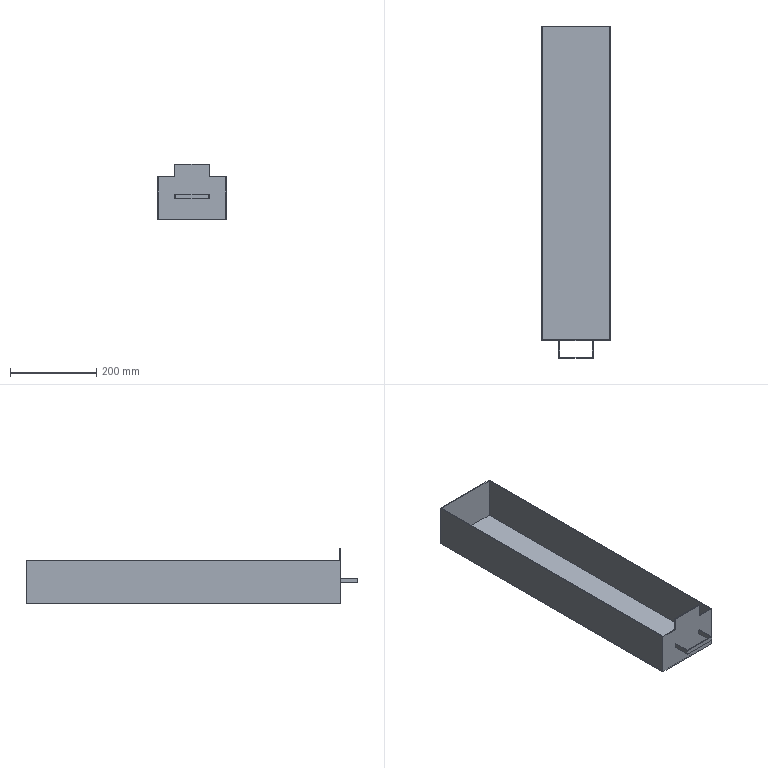Part | NX | features solid 2 | 1 solid | 22 faces | box 160 x 772 x 130 mm | volume 590256 mm3 | plane 22
STEP:
#1=CARTESIAN_POINT('',(-175.,-255.,-465.));
#2=VERTEX_POINT('',#1);
#3=CARTESIAN_POINT('',(-175.,-987.,-465.));
#4=VERTEX_POINT('',#3);
#5=CARTESIAN_POINT('',(-175.,-687.,-465.));
#6=DIRECTION('',(0.,-1.,0.));
#7=VECTOR('',#6,1000.);
#8=LINE('',#5,#7);
#9=EDGE_CURVE('',#2,#4,#8,.T.);
#10=ORIENTED_EDGE('',*,*,#9,.T.);
#11=CARTESIAN_POINT('',(-175.,-987.,-565.));
#12=VERTEX_POINT('',#11);
#13=CARTESIAN_POINT('',(-175.,-987.,-565.));
#14=DIRECTION('',(0.,0.,1.));
#15=VECTOR('',#14,1000.);
#16=LINE('',#13,#15);
#17=EDGE_CURVE('',#12,#4,#16,.T.);
#18=ORIENTED_EDGE('',*,*,#17,.F.);
#19=CARTESIAN_POINT('',(-175.,-255.,-565.));
#20=VERTEX_POINT('',#19);
#21=CARTESIAN_POINT('',(-175.,-687.,-565.));
#22=DIRECTION('',(0.,-1.,0.));
#23=VECTOR('',#22,1000.);
#24=LINE('',#21,#23);
#25=EDGE_CURVE('',#20,#12,#24,.T.);
#26=ORIENTED_EDGE('',*,*,#25,.F.);
#27=CARTESIAN_POINT('',(-175.,-255.,-565.));
#28=DIRECTION('',(0.,0.,-1.));
#29=VECTOR('',#28,1000.);
#30=LINE('',#27,#29);
#31=EDGE_CURVE('',#20,#2,#30,.F.);
#32=ORIENTED_EDGE('',*,*,#31,.T.);
#33=EDGE_LOOP('',(#10,#18,#26,#32));
#34=FACE_BOUND('',#33,.T.);
#35=CARTESIAN_POINT('',(-175.,-687.,-565.));
#36=DIRECTION('',(-1.,0.,0.));
#37=DIRECTION('',(0.,-1.,0.));
#38=AXIS2_PLACEMENT_3D('',#35,#36,#37);
#39=PLANE('',#38);
#40=ADVANCED_FACE('',(#34),#39,.F.);
#41=CARTESIAN_POINT('',(-295.,-987.,-505.));
#42=VERTEX_POINT('',#41);
#43=CARTESIAN_POINT('',(-295.,-987.,-515.));
#44=VERTEX_POINT('',#43);
#45=CARTESIAN_POINT('',(-295.,-987.,-565.));
#46=DIRECTION('',(0.,0.,-1.));
#47=VECTOR('',#46,1000.);
#48=LINE('',#45,#47);
#49=EDGE_CURVE('',#42,#44,#48,.T.);
#50=ORIENTED_EDGE('',*,*,#49,.F.);
#51=CARTESIAN_POINT('',(-293.,-987.,-505.));
#52=VERTEX_POINT('',#51);
#53=CARTESIAN_POINT('',(-215.,-987.,-505.));
#54=DIRECTION('',(1.,0.,0.));
#55=VECTOR('',#54,1000.);
#56=LINE('',#53,#55);
#57=EDGE_CURVE('',#52,#42,#56,.F.);
#58=ORIENTED_EDGE('',*,*,#57,.F.);
#59=CARTESIAN_POINT('',(-293.,-987.,-515.));
#60=VERTEX_POINT('',#59);
#61=CARTESIAN_POINT('',(-293.,-987.,-565.));
#62=DIRECTION('',(0.,0.,-1.));
#63=VECTOR('',#62,1000.);
#64=LINE('',#61,#63);
#65=EDGE_CURVE('',#52,#60,#64,.T.);
#66=ORIENTED_EDGE('',*,*,#65,.T.);
#67=CARTESIAN_POINT('',(-215.,-987.,-515.));
#68=DIRECTION('',(1.,0.,0.));
#69=VECTOR('',#68,1000.);
#70=LINE('',#67,#69);
#71=EDGE_CURVE('',#60,#44,#70,.F.);
#72=ORIENTED_EDGE('',*,*,#71,.T.);
#73=EDGE_LOOP('',(#50,#58,#66,#72));
#74=FACE_BOUND('',#73,.T.);
#75=CARTESIAN_POINT('',(-217.,-987.,-505.));
#76=VERTEX_POINT('',#75);
#77=CARTESIAN_POINT('',(-217.,-987.,-515.));
#78=VERTEX_POINT('',#77);
#79=CARTESIAN_POINT('',(-217.,-987.,-565.));
#80=DIRECTION('',(0.,0.,1.));
#81=VECTOR('',#80,1000.);
#82=LINE('',#79,#81);
#83=EDGE_CURVE('',#76,#78,#82,.F.);
#84=ORIENTED_EDGE('',*,*,#83,.F.);
#85=CARTESIAN_POINT('',(-215.,-987.,-505.));
#86=VERTEX_POINT('',#85);
#87=CARTESIAN_POINT('',(-215.,-987.,-505.));
#88=DIRECTION('',(1.,0.,0.));
#89=VECTOR('',#88,1000.);
#90=LINE('',#87,#89);
#91=EDGE_CURVE('',#86,#76,#90,.F.);
#92=ORIENTED_EDGE('',*,*,#91,.F.);
#93=CARTESIAN_POINT('',(-215.,-987.,-515.));
#94=VERTEX_POINT('',#93);
#95=CARTESIAN_POINT('',(-215.,-987.,-565.));
#96=DIRECTION('',(0.,0.,-1.));
#97=VECTOR('',#96,1000.);
#98=LINE('',#95,#97);
#99=EDGE_CURVE('',#86,#94,#98,.T.);
#100=ORIENTED_EDGE('',*,*,#99,.T.);
#101=CARTESIAN_POINT('',(-215.,-987.,-515.));
#102=DIRECTION('',(1.,0.,0.));
#103=VECTOR('',#102,1000.);
#104=LINE('',#101,#103);
#105=EDGE_CURVE('',#94,#78,#104,.F.);
#106=ORIENTED_EDGE('',*,*,#105,.T.);
#107=EDGE_LOOP('',(#84,#92,#100,#106));
#108=FACE_BOUND('',#107,.T.);
#109=CARTESIAN_POINT('',(-335.,-987.,-465.));
#110=VERTEX_POINT('',#109);
#111=CARTESIAN_POINT('',(-295.,-987.,-465.));
#112=VERTEX_POINT('',#111);
#113=CARTESIAN_POINT('',(-180.,-987.,-465.));
#114=DIRECTION('',(1.,0.,0.));
#115=VECTOR('',#114,1000.);
#116=LINE('',#113,#115);
#117=EDGE_CURVE('',#110,#112,#116,.T.);
#118=ORIENTED_EDGE('',*,*,#117,.F.);
#119=CARTESIAN_POINT('',(-335.,-987.,-565.));
#120=VERTEX_POINT('',#119);
#121=CARTESIAN_POINT('',(-335.,-987.,-565.));
#122=DIRECTION('',(0.,0.,-1.));
#123=VECTOR('',#122,1000.);
#124=LINE('',#121,#123);
#125=EDGE_CURVE('',#120,#110,#124,.F.);
#126=ORIENTED_EDGE('',*,*,#125,.F.);
#127=CARTESIAN_POINT('',(-180.,-987.,-565.));
#128=DIRECTION('',(-1.,0.,0.));
#129=VECTOR('',#128,1000.);
#130=LINE('',#127,#129);
#131=EDGE_CURVE('',#12,#120,#130,.T.);
#132=ORIENTED_EDGE('',*,*,#131,.F.);
#133=ORIENTED_EDGE('',*,*,#17,.T.);
#134=CARTESIAN_POINT('',(-215.,-987.,-465.));
#135=VERTEX_POINT('',#134);
#136=CARTESIAN_POINT('',(-180.,-987.,-465.));
#137=DIRECTION('',(1.,0.,0.));
#138=VECTOR('',#137,1000.);
#139=LINE('',#136,#138);
#140=EDGE_CURVE('',#135,#4,#139,.T.);
#141=ORIENTED_EDGE('',*,*,#140,.F.);
#142=CARTESIAN_POINT('',(-215.,-987.,-435.));
#143=VERTEX_POINT('',#142);
#144=CARTESIAN_POINT('',(-215.,-987.,-565.));
#145=DIRECTION('',(0.,0.,1.));
#146=VECTOR('',#145,1000.);
#147=LINE('',#144,#146);
#148=EDGE_CURVE('',#135,#143,#147,.T.);
#149=ORIENTED_EDGE('',*,*,#148,.T.);
#150=CARTESIAN_POINT('',(-295.,-987.,-435.));
#151=VERTEX_POINT('',#150);
#152=CARTESIAN_POINT('',(-175.,-987.,-435.));
#153=DIRECTION('',(-1.,0.,0.));
#154=VECTOR('',#153,1000.);
#155=LINE('',#152,#154);
#156=EDGE_CURVE('',#143,#151,#155,.T.);
#157=ORIENTED_EDGE('',*,*,#156,.T.);
#158=CARTESIAN_POINT('',(-295.,-987.,-565.));
#159=DIRECTION('',(0.,0.,-1.));
#160=VECTOR('',#159,1000.);
#161=LINE('',#158,#160);
#162=EDGE_CURVE('',#112,#151,#161,.F.);
#163=ORIENTED_EDGE('',*,*,#162,.F.);
#164=EDGE_LOOP('',(#118,#126,#132,#133,#141,#149,#157,#163));
#165=FACE_BOUND('',#164,.T.);
#166=CARTESIAN_POINT('',(-180.,-987.,-565.));
#167=DIRECTION('',(0.,1.,0.));
#168=DIRECTION('',(-1.,0.,0.));
#169=AXIS2_PLACEMENT_3D('',#166,#167,#168);
#170=PLANE('',#169);
#171=ADVANCED_FACE('',(#74,#108,#165),#170,.F.);
#172=ORIENTED_EDGE('',*,*,#125,.T.);
#173=CARTESIAN_POINT('',(-335.,-255.,-465.));
#174=VERTEX_POINT('',#173);
#175=CARTESIAN_POINT('',(-335.,-687.,-465.));
#176=DIRECTION('',(0.,1.,0.));
#177=VECTOR('',#176,1000.);
#178=LINE('',#175,#177);
#179=EDGE_CURVE('',#174,#110,#178,.F.);
#180=ORIENTED_EDGE('',*,*,#179,.F.);
#181=CARTESIAN_POINT('',(-335.,-255.,-565.));
#182=VERTEX_POINT('',#181);
#183=CARTESIAN_POINT('',(-335.,-255.,-565.));
#184=DIRECTION('',(0.,0.,1.));
#185=VECTOR('',#184,1000.);
#186=LINE('',#183,#185);
#187=EDGE_CURVE('',#182,#174,#186,.T.);
#188=ORIENTED_EDGE('',*,*,#187,.F.);
#189=CARTESIAN_POINT('',(-335.,-687.,-565.));
#190=DIRECTION('',(0.,1.,0.));
#191=VECTOR('',#190,1000.);
#192=LINE('',#189,#191);
#193=EDGE_CURVE('',#182,#120,#192,.F.);
#194=ORIENTED_EDGE('',*,*,#193,.T.);
#195=EDGE_LOOP('',(#172,#180,#188,#194));
#196=FACE_BOUND('',#195,.T.);
#197=CARTESIAN_POINT('',(-335.,-687.,-565.));
#198=DIRECTION('',(-1.,0.,0.));
#199=DIRECTION('',(0.,-1.,0.));
#200=AXIS2_PLACEMENT_3D('',#197,#198,#199);
#201=PLANE('',#200);
#202=ADVANCED_FACE('',(#196),#201,.T.);
#203=CARTESIAN_POINT('',(-333.,-985.,-563.));
#204=VERTEX_POINT('',#203);
#205=CARTESIAN_POINT('',(-333.,-985.,-465.));
#206=VERTEX_POINT('',#205);
#207=CARTESIAN_POINT('',(-333.,-985.,-565.));
#208=DIRECTION('',(0.,0.,-1.));
#209=VECTOR('',#208,1000.);
#210=LINE('',#207,#209);
#211=EDGE_CURVE('',#204,#206,#210,.F.);
#212=ORIENTED_EDGE('',*,*,#211,.T.);
#213=CARTESIAN_POINT('',(-295.,-985.,-465.));
#214=VERTEX_POINT('',#213);
#215=CARTESIAN_POINT('',(-180.,-985.,-465.));
#216=DIRECTION('',(1.,0.,0.));
#217=VECTOR('',#216,1000.);
#218=LINE('',#215,#217);
#219=EDGE_CURVE('',#206,#214,#218,.T.);
#220=ORIENTED_EDGE('',*,*,#219,.T.);
#221=CARTESIAN_POINT('',(-295.,-985.,-435.));
#222=VERTEX_POINT('',#221);
#223=CARTESIAN_POINT('',(-295.,-985.,-565.));
#224=DIRECTION('',(0.,0.,-1.));
#225=VECTOR('',#224,1000.);
#226=LINE('',#223,#225);
#227=EDGE_CURVE('',#214,#222,#226,.F.);
#228=ORIENTED_EDGE('',*,*,#227,.T.);
#229=CARTESIAN_POINT('',(-215.,-985.,-435.));
#230=VERTEX_POINT('',#229);
#231=CARTESIAN_POINT('',(-175.,-985.,-435.));
#232=DIRECTION('',(-1.,0.,0.));
#233=VECTOR('',#232,1000.);
#234=LINE('',#231,#233);
#235=EDGE_CURVE('',#230,#222,#234,.T.);
#236=ORIENTED_EDGE('',*,*,#235,.F.);
#237=CARTESIAN_POINT('',(-215.,-985.,-465.));
#238=VERTEX_POINT('',#237);
#239=CARTESIAN_POINT('',(-215.,-985.,-565.));
#240=DIRECTION('',(0.,0.,1.));
#241=VECTOR('',#240,1000.);
#242=LINE('',#239,#241);
#243=EDGE_CURVE('',#238,#230,#242,.T.);
#244=ORIENTED_EDGE('',*,*,#243,.F.);
#245=CARTESIAN_POINT('',(-177.,-985.,-465.));
#246=VERTEX_POINT('',#245);
#247=CARTESIAN_POINT('',(-180.,-985.,-465.));
#248=DIRECTION('',(1.,0.,0.));
#249=VECTOR('',#248,1000.);
#250=LINE('',#247,#249);
#251=EDGE_CURVE('',#238,#246,#250,.T.);
#252=ORIENTED_EDGE('',*,*,#251,.T.);
#253=CARTESIAN_POINT('',(-177.,-985.,-563.));
#254=VERTEX_POINT('',#253);
#255=CARTESIAN_POINT('',(-177.,-985.,-565.));
#256=DIRECTION('',(0.,0.,1.));
#257=VECTOR('',#256,1000.);
#258=LINE('',#255,#257);
#259=EDGE_CURVE('',#254,#246,#258,.T.);
#260=ORIENTED_EDGE('',*,*,#259,.F.);
#261=CARTESIAN_POINT('',(-180.,-985.,-563.));
#262=DIRECTION('',(-1.,0.,0.));
#263=VECTOR('',#262,1000.);
#264=LINE('',#261,#263);
#265=EDGE_CURVE('',#254,#204,#264,.T.);
#266=ORIENTED_EDGE('',*,*,#265,.T.);
#267=EDGE_LOOP('',(#212,#220,#228,#236,#244,#252,#260,#266));
#268=FACE_BOUND('',#267,.T.);
#269=CARTESIAN_POINT('',(-180.,-985.,-565.));
#270=DIRECTION('',(0.,1.,0.));
#271=DIRECTION('',(-1.,0.,0.));
#272=AXIS2_PLACEMENT_3D('',#269,#270,#271);
#273=PLANE('',#272);
#274=ADVANCED_FACE('',(#268),#273,.T.);
#275=CARTESIAN_POINT('',(-295.,-687.,-465.));
#276=DIRECTION('',(0.,1.,0.));
#277=VECTOR('',#276,1000.);
#278=LINE('',#275,#277);
#279=EDGE_CURVE('',#214,#112,#278,.F.);
#280=ORIENTED_EDGE('',*,*,#279,.F.);
#281=ORIENTED_EDGE('',*,*,#219,.F.);
#282=CARTESIAN_POINT('',(-333.,-257.,-465.));
#283=VERTEX_POINT('',#282);
#284=CARTESIAN_POINT('',(-333.,-687.,-465.));
#285=DIRECTION('',(0.,1.,0.));
#286=VECTOR('',#285,1000.);
#287=LINE('',#284,#286);
#288=EDGE_CURVE('',#283,#206,#287,.F.);
#289=ORIENTED_EDGE('',*,*,#288,.F.);
#290=CARTESIAN_POINT('',(-177.,-257.,-465.));
#291=VERTEX_POINT('',#290);
#292=CARTESIAN_POINT('',(-180.,-257.,-465.));
#293=DIRECTION('',(1.,0.,0.));
#294=VECTOR('',#293,1000.);
#295=LINE('',#292,#294);
#296=EDGE_CURVE('',#291,#283,#295,.F.);
#297=ORIENTED_EDGE('',*,*,#296,.F.);
#298=CARTESIAN_POINT('',(-177.,-687.,-465.));
#299=DIRECTION('',(0.,-1.,0.));
#300=VECTOR('',#299,1000.);
#301=LINE('',#298,#300);
#302=EDGE_CURVE('',#291,#246,#301,.T.);
#303=ORIENTED_EDGE('',*,*,#302,.T.);
#304=ORIENTED_EDGE('',*,*,#251,.F.);
#305=CARTESIAN_POINT('',(-215.,-687.,-465.));
#306=DIRECTION('',(0.,1.,0.));
#307=VECTOR('',#306,1000.);
#308=LINE('',#305,#307);
#309=EDGE_CURVE('',#135,#238,#308,.T.);
#310=ORIENTED_EDGE('',*,*,#309,.F.);
#311=ORIENTED_EDGE('',*,*,#140,.T.);
#312=ORIENTED_EDGE('',*,*,#9,.F.);
#313=CARTESIAN_POINT('',(-180.,-255.,-465.));
#314=DIRECTION('',(1.,0.,0.));
#315=VECTOR('',#314,1000.);
#316=LINE('',#313,#315);
#317=EDGE_CURVE('',#2,#174,#316,.F.);
#318=ORIENTED_EDGE('',*,*,#317,.T.);
#319=ORIENTED_EDGE('',*,*,#179,.T.);
#320=ORIENTED_EDGE('',*,*,#117,.T.);
#321=EDGE_LOOP('',(#280,#281,#289,#297,#303,#304,#310,#311,#312,#318,#319,#320));
#322=FACE_BOUND('',#321,.T.);
#323=CARTESIAN_POINT('',(-180.,-687.,-465.));
#324=DIRECTION('',(0.,0.,1.));
#325=DIRECTION('',(1.,0.,0.));
#326=AXIS2_PLACEMENT_3D('',#323,#324,#325);
#327=PLANE('',#326);
#328=ADVANCED_FACE('',(#322),#327,.T.);
#329=ORIENTED_EDGE('',*,*,#187,.T.);
#330=ORIENTED_EDGE('',*,*,#317,.F.);
#331=ORIENTED_EDGE('',*,*,#31,.F.);
#332=CARTESIAN_POINT('',(-180.,-255.,-565.));
#333=DIRECTION('',(1.,0.,0.));
#334=VECTOR('',#333,1000.);
#335=LINE('',#332,#334);
#336=EDGE_CURVE('',#20,#182,#335,.F.);
#337=ORIENTED_EDGE('',*,*,#336,.T.);
#338=EDGE_LOOP('',(#329,#330,#331,#337));
#339=FACE_BOUND('',#338,.T.);
#340=CARTESIAN_POINT('',(-180.,-255.,-565.));
#341=DIRECTION('',(0.,1.,0.));
#342=DIRECTION('',(-1.,0.,0.));
#343=AXIS2_PLACEMENT_3D('',#340,#341,#342);
#344=PLANE('',#343);
#345=ADVANCED_FACE('',(#339),#344,.T.);
#346=ORIENTED_EDGE('',*,*,#131,.T.);
#347=ORIENTED_EDGE('',*,*,#193,.F.);
#348=ORIENTED_EDGE('',*,*,#336,.F.);
#349=ORIENTED_EDGE('',*,*,#25,.T.);
#350=EDGE_LOOP('',(#346,#347,#348,#349));
#351=FACE_BOUND('',#350,.T.);
#352=CARTESIAN_POINT('',(-180.,-687.,-565.));
#353=DIRECTION('',(0.,0.,1.));
#354=DIRECTION('',(1.,0.,0.));
#355=AXIS2_PLACEMENT_3D('',#352,#353,#354);
#356=PLANE('',#355);
#357=ADVANCED_FACE('',(#351),#356,.F.);
#358=CARTESIAN_POINT('',(-333.,-257.,-563.));
#359=VERTEX_POINT('',#358);
#360=CARTESIAN_POINT('',(-333.,-257.,-565.));
#361=DIRECTION('',(0.,0.,1.));
#362=VECTOR('',#361,1000.);
#363=LINE('',#360,#362);
#364=EDGE_CURVE('',#359,#283,#363,.T.);
#365=ORIENTED_EDGE('',*,*,#364,.F.);
#366=CARTESIAN_POINT('',(-177.,-257.,-563.));
#367=VERTEX_POINT('',#366);
#368=CARTESIAN_POINT('',(-180.,-257.,-563.));
#369=DIRECTION('',(1.,0.,0.));
#370=VECTOR('',#369,1000.);
#371=LINE('',#368,#370);
#372=EDGE_CURVE('',#367,#359,#371,.F.);
#373=ORIENTED_EDGE('',*,*,#372,.F.);
#374=CARTESIAN_POINT('',(-177.,-257.,-565.));
#375=DIRECTION('',(0.,0.,-1.));
#376=VECTOR('',#375,1000.);
#377=LINE('',#374,#376);
#378=EDGE_CURVE('',#367,#291,#377,.F.);
#379=ORIENTED_EDGE('',*,*,#378,.T.);
#380=ORIENTED_EDGE('',*,*,#296,.T.);
#381=EDGE_LOOP('',(#365,#373,#379,#380));
#382=FACE_BOUND('',#381,.T.);
#383=CARTESIAN_POINT('',(-180.,-257.,-565.));
#384=DIRECTION('',(0.,1.,0.));
#385=DIRECTION('',(-1.,0.,0.));
#386=AXIS2_PLACEMENT_3D('',#383,#384,#385);
#387=PLANE('',#386);
#388=ADVANCED_FACE('',(#382),#387,.F.);
#389=ORIENTED_EDGE('',*,*,#378,.F.);
#390=CARTESIAN_POINT('',(-177.,-687.,-563.));
#391=DIRECTION('',(0.,-1.,0.));
#392=VECTOR('',#391,1000.);
#393=LINE('',#390,#392);
#394=EDGE_CURVE('',#367,#254,#393,.T.);
#395=ORIENTED_EDGE('',*,*,#394,.T.);
#396=ORIENTED_EDGE('',*,*,#259,.T.);
#397=ORIENTED_EDGE('',*,*,#302,.F.);
#398=EDGE_LOOP('',(#389,#395,#396,#397));
#399=FACE_BOUND('',#398,.T.);
#400=CARTESIAN_POINT('',(-177.,-687.,-565.));
#401=DIRECTION('',(-1.,0.,0.));
#402=DIRECTION('',(0.,-1.,0.));
#403=AXIS2_PLACEMENT_3D('',#400,#401,#402);
#404=PLANE('',#403);
#405=ADVANCED_FACE('',(#399),#404,.T.);
#406=CARTESIAN_POINT('',(-333.,-687.,-563.));
#407=DIRECTION('',(0.,1.,0.));
#408=VECTOR('',#407,1000.);
#409=LINE('',#406,#408);
#410=EDGE_CURVE('',#359,#204,#409,.F.);
#411=ORIENTED_EDGE('',*,*,#410,.F.);
#412=ORIENTED_EDGE('',*,*,#364,.T.);
#413=ORIENTED_EDGE('',*,*,#288,.T.);
#414=ORIENTED_EDGE('',*,*,#211,.F.);
#415=EDGE_LOOP('',(#411,#412,#413,#414));
#416=FACE_BOUND('',#415,.T.);
#417=CARTESIAN_POINT('',(-333.,-687.,-565.));
#418=DIRECTION('',(-1.,0.,0.));
#419=DIRECTION('',(0.,-1.,0.));
#420=AXIS2_PLACEMENT_3D('',#417,#418,#419);
#421=PLANE('',#420);
#422=ADVANCED_FACE('',(#416),#421,.F.);
#423=ORIENTED_EDGE('',*,*,#265,.F.);
#424=ORIENTED_EDGE('',*,*,#394,.F.);
#425=ORIENTED_EDGE('',*,*,#372,.T.);
#426=ORIENTED_EDGE('',*,*,#410,.T.);
#427=EDGE_LOOP('',(#423,#424,#425,#426));
#428=FACE_BOUND('',#427,.T.);
#429=CARTESIAN_POINT('',(-180.,-687.,-563.));
#430=DIRECTION('',(0.,0.,1.));
#431=DIRECTION('',(1.,0.,0.));
#432=AXIS2_PLACEMENT_3D('',#429,#430,#431);
#433=PLANE('',#432);
#434=ADVANCED_FACE('',(#428),#433,.T.);
#435=ORIENTED_EDGE('',*,*,#91,.T.);
#436=CARTESIAN_POINT('',(-217.,-1025.,-505.));
#437=VERTEX_POINT('',#436);
#438=CARTESIAN_POINT('',(-217.,-987.,-505.));
#439=DIRECTION('',(0.,1.,0.));
#440=VECTOR('',#439,1000.);
#441=LINE('',#438,#440);
#442=EDGE_CURVE('',#76,#437,#441,.F.);
#443=ORIENTED_EDGE('',*,*,#442,.T.);
#444=CARTESIAN_POINT('',(-293.,-1025.,-505.));
#445=VERTEX_POINT('',#444);
#446=CARTESIAN_POINT('',(-215.,-1025.,-505.));
#447=DIRECTION('',(1.,0.,0.));
#448=VECTOR('',#447,1000.);
#449=LINE('',#446,#448);
#450=EDGE_CURVE('',#437,#445,#449,.F.);
#451=ORIENTED_EDGE('',*,*,#450,.T.);
#452=CARTESIAN_POINT('',(-293.,-987.,-505.));
#453=DIRECTION('',(0.,-1.,0.));
#454=VECTOR('',#453,1000.);
#455=LINE('',#452,#454);
#456=EDGE_CURVE('',#52,#445,#455,.T.);
#457=ORIENTED_EDGE('',*,*,#456,.F.);
#458=ORIENTED_EDGE('',*,*,#57,.T.);
#459=CARTESIAN_POINT('',(-295.,-1027.,-505.));
#460=VERTEX_POINT('',#459);
#461=CARTESIAN_POINT('',(-295.,-987.,-505.));
#462=DIRECTION('',(0.,1.,0.));
#463=VECTOR('',#462,1000.);
#464=LINE('',#461,#463);
#465=EDGE_CURVE('',#42,#460,#464,.F.);
#466=ORIENTED_EDGE('',*,*,#465,.T.);
#467=CARTESIAN_POINT('',(-215.,-1027.,-505.));
#468=VERTEX_POINT('',#467);
#469=CARTESIAN_POINT('',(-215.,-1027.,-505.));
#470=DIRECTION('',(1.,0.,0.));
#471=VECTOR('',#470,1000.);
#472=LINE('',#469,#471);
#473=EDGE_CURVE('',#468,#460,#472,.F.);
#474=ORIENTED_EDGE('',*,*,#473,.F.);
#475=CARTESIAN_POINT('',(-215.,-987.,-505.));
#476=DIRECTION('',(0.,1.,0.));
#477=VECTOR('',#476,1000.);
#478=LINE('',#475,#477);
#479=EDGE_CURVE('',#86,#468,#478,.F.);
#480=ORIENTED_EDGE('',*,*,#479,.F.);
#481=EDGE_LOOP('',(#435,#443,#451,#457,#458,#466,#474,#480));
#482=FACE_BOUND('',#481,.T.);
#483=CARTESIAN_POINT('',(-215.,-987.,-505.));
#484=DIRECTION('',(0.,0.,1.));
#485=DIRECTION('',(1.,0.,0.));
#486=AXIS2_PLACEMENT_3D('',#483,#484,#485);
#487=PLANE('',#486);
#488=ADVANCED_FACE('',(#482),#487,.T.);
#489=ORIENTED_EDGE('',*,*,#99,.F.);
#490=ORIENTED_EDGE('',*,*,#479,.T.);
#491=CARTESIAN_POINT('',(-215.,-1027.,-515.));
#492=VERTEX_POINT('',#491);
#493=CARTESIAN_POINT('',(-215.,-1027.,-565.));
#494=DIRECTION('',(0.,0.,-1.));
#495=VECTOR('',#494,1000.);
#496=LINE('',#493,#495);
#497=EDGE_CURVE('',#468,#492,#496,.T.);
#498=ORIENTED_EDGE('',*,*,#497,.T.);
#499=CARTESIAN_POINT('',(-215.,-987.,-515.));
#500=DIRECTION('',(0.,1.,0.));
#501=VECTOR('',#500,1000.);
#502=LINE('',#499,#501);
#503=EDGE_CURVE('',#94,#492,#502,.F.);
#504=ORIENTED_EDGE('',*,*,#503,.F.);
#505=EDGE_LOOP('',(#489,#490,#498,#504));
#506=FACE_BOUND('',#505,.T.);
#507=CARTESIAN_POINT('',(-215.,-987.,-565.));
#508=DIRECTION('',(-1.,0.,0.));
#509=DIRECTION('',(0.,-1.,0.));
#510=AXIS2_PLACEMENT_3D('',#507,#508,#509);
#511=PLANE('',#510);
#512=ADVANCED_FACE('',(#506),#511,.F.);
#513=ORIENTED_EDGE('',*,*,#497,.F.);
#514=ORIENTED_EDGE('',*,*,#473,.T.);
#515=CARTESIAN_POINT('',(-295.,-1027.,-515.));
#516=VERTEX_POINT('',#515);
#517=CARTESIAN_POINT('',(-295.,-1027.,-565.));
#518=DIRECTION('',(0.,0.,-1.));
#519=VECTOR('',#518,1000.);
#520=LINE('',#517,#519);
#521=EDGE_CURVE('',#460,#516,#520,.T.);
#522=ORIENTED_EDGE('',*,*,#521,.T.);
#523=CARTESIAN_POINT('',(-215.,-1027.,-515.));
#524=DIRECTION('',(1.,0.,0.));
#525=VECTOR('',#524,1000.);
#526=LINE('',#523,#525);
#527=EDGE_CURVE('',#492,#516,#526,.F.);
#528=ORIENTED_EDGE('',*,*,#527,.F.);
#529=EDGE_LOOP('',(#513,#514,#522,#528));
#530=FACE_BOUND('',#529,.T.);
#531=CARTESIAN_POINT('',(-215.,-1027.,-565.));
#532=DIRECTION('',(0.,1.,0.));
#533=DIRECTION('',(-1.,0.,0.));
#534=AXIS2_PLACEMENT_3D('',#531,#532,#533);
#535=PLANE('',#534);
#536=ADVANCED_FACE('',(#530),#535,.F.);
#537=ORIENTED_EDGE('',*,*,#71,.F.);
#538=CARTESIAN_POINT('',(-293.,-1025.,-515.));
#539=VERTEX_POINT('',#538);
#540=CARTESIAN_POINT('',(-293.,-987.,-515.));
#541=DIRECTION('',(0.,-1.,0.));
#542=VECTOR('',#541,1000.);
#543=LINE('',#540,#542);
#544=EDGE_CURVE('',#60,#539,#543,.T.);
#545=ORIENTED_EDGE('',*,*,#544,.T.);
#546=CARTESIAN_POINT('',(-217.,-1025.,-515.));
#547=VERTEX_POINT('',#546);
#548=CARTESIAN_POINT('',(-215.,-1025.,-515.));
#549=DIRECTION('',(1.,0.,0.));
#550=VECTOR('',#549,1000.);
#551=LINE('',#548,#550);
#552=EDGE_CURVE('',#547,#539,#551,.F.);
#553=ORIENTED_EDGE('',*,*,#552,.F.);
#554=CARTESIAN_POINT('',(-217.,-987.,-515.));
#555=DIRECTION('',(0.,1.,0.));
#556=VECTOR('',#555,1000.);
#557=LINE('',#554,#556);
#558=EDGE_CURVE('',#78,#547,#557,.F.);
#559=ORIENTED_EDGE('',*,*,#558,.F.);
#560=ORIENTED_EDGE('',*,*,#105,.F.);
#561=ORIENTED_EDGE('',*,*,#503,.T.);
#562=ORIENTED_EDGE('',*,*,#527,.T.);
#563=CARTESIAN_POINT('',(-295.,-987.,-515.));
#564=DIRECTION('',(0.,1.,0.));
#565=VECTOR('',#564,1000.);
#566=LINE('',#563,#565);
#567=EDGE_CURVE('',#44,#516,#566,.F.);
#568=ORIENTED_EDGE('',*,*,#567,.F.);
#569=EDGE_LOOP('',(#537,#545,#553,#559,#560,#561,#562,#568));
#570=FACE_BOUND('',#569,.T.);
#571=CARTESIAN_POINT('',(-215.,-987.,-515.));
#572=DIRECTION('',(0.,0.,1.));
#573=DIRECTION('',(1.,0.,0.));
#574=AXIS2_PLACEMENT_3D('',#571,#572,#573);
#575=PLANE('',#574);
#576=ADVANCED_FACE('',(#570),#575,.F.);
#577=ORIENTED_EDGE('',*,*,#465,.F.);
#578=ORIENTED_EDGE('',*,*,#49,.T.);
#579=ORIENTED_EDGE('',*,*,#567,.T.);
#580=ORIENTED_EDGE('',*,*,#521,.F.);
#581=EDGE_LOOP('',(#577,#578,#579,#580));
#582=FACE_BOUND('',#581,.T.);
#583=CARTESIAN_POINT('',(-295.,-987.,-565.));
#584=DIRECTION('',(-1.,0.,0.));
#585=DIRECTION('',(0.,-1.,0.));
#586=AXIS2_PLACEMENT_3D('',#583,#584,#585);
#587=PLANE('',#586);
#588=ADVANCED_FACE('',(#582),#587,.T.);
#589=ORIENTED_EDGE('',*,*,#83,.T.);
#590=ORIENTED_EDGE('',*,*,#558,.T.);
#591=CARTESIAN_POINT('',(-217.,-1025.,-565.));
#592=DIRECTION('',(0.,0.,-1.));
#593=VECTOR('',#592,1000.);
#594=LINE('',#591,#593);
#595=EDGE_CURVE('',#437,#547,#594,.T.);
#596=ORIENTED_EDGE('',*,*,#595,.F.);
#597=ORIENTED_EDGE('',*,*,#442,.F.);
#598=EDGE_LOOP('',(#589,#590,#596,#597));
#599=FACE_BOUND('',#598,.T.);
#600=CARTESIAN_POINT('',(-217.,-987.,-565.));
#601=DIRECTION('',(-1.,0.,0.));
#602=DIRECTION('',(0.,-1.,0.));
#603=AXIS2_PLACEMENT_3D('',#600,#601,#602);
#604=PLANE('',#603);
#605=ADVANCED_FACE('',(#599),#604,.T.);
#606=ORIENTED_EDGE('',*,*,#595,.T.);
#607=ORIENTED_EDGE('',*,*,#552,.T.);
#608=CARTESIAN_POINT('',(-293.,-1025.,-565.));
#609=DIRECTION('',(0.,0.,1.));
#610=VECTOR('',#609,1000.);
#611=LINE('',#608,#610);
#612=EDGE_CURVE('',#445,#539,#611,.F.);
#613=ORIENTED_EDGE('',*,*,#612,.F.);
#614=ORIENTED_EDGE('',*,*,#450,.F.);
#615=EDGE_LOOP('',(#606,#607,#613,#614));
#616=FACE_BOUND('',#615,.T.);
#617=CARTESIAN_POINT('',(-215.,-1025.,-565.));
#618=DIRECTION('',(0.,1.,0.));
#619=DIRECTION('',(-1.,0.,0.));
#620=AXIS2_PLACEMENT_3D('',#617,#618,#619);
#621=PLANE('',#620);
#622=ADVANCED_FACE('',(#616),#621,.T.);
#623=ORIENTED_EDGE('',*,*,#456,.T.);
#624=ORIENTED_EDGE('',*,*,#612,.T.);
#625=ORIENTED_EDGE('',*,*,#544,.F.);
#626=ORIENTED_EDGE('',*,*,#65,.F.);
#627=EDGE_LOOP('',(#623,#624,#625,#626));
#628=FACE_BOUND('',#627,.T.);
#629=CARTESIAN_POINT('',(-293.,-987.,-565.));
#630=DIRECTION('',(-1.,0.,0.));
#631=DIRECTION('',(0.,-1.,0.));
#632=AXIS2_PLACEMENT_3D('',#629,#630,#631);
#633=PLANE('',#632);
#634=ADVANCED_FACE('',(#628),#633,.F.);
#635=ORIENTED_EDGE('',*,*,#235,.T.);
#636=CARTESIAN_POINT('',(-295.,-687.,-435.));
#637=DIRECTION('',(0.,-1.,0.));
#638=VECTOR('',#637,1000.);
#639=LINE('',#636,#638);
#640=EDGE_CURVE('',#151,#222,#639,.F.);
#641=ORIENTED_EDGE('',*,*,#640,.F.);
#642=ORIENTED_EDGE('',*,*,#156,.F.);
#643=CARTESIAN_POINT('',(-215.,-987.,-435.));
#644=DIRECTION('',(0.,1.,0.));
#645=VECTOR('',#644,1000.);
#646=LINE('',#643,#645);
#647=EDGE_CURVE('',#143,#230,#646,.T.);
#648=ORIENTED_EDGE('',*,*,#647,.T.);
#649=EDGE_LOOP('',(#635,#641,#642,#648));
#650=FACE_BOUND('',#649,.T.);
#651=CARTESIAN_POINT('',(-175.,-987.,-435.));
#652=DIRECTION('',(0.,0.,-1.));
#653=DIRECTION('',(-1.,0.,0.));
#654=AXIS2_PLACEMENT_3D('',#651,#652,#653);
#655=PLANE('',#654);
#656=ADVANCED_FACE('',(#650),#655,.F.);
#657=ORIENTED_EDGE('',*,*,#227,.F.);
#658=ORIENTED_EDGE('',*,*,#279,.T.);
#659=ORIENTED_EDGE('',*,*,#162,.T.);
#660=ORIENTED_EDGE('',*,*,#640,.T.);
#661=EDGE_LOOP('',(#657,#658,#659,#660));
#662=FACE_BOUND('',#661,.T.);
#663=CARTESIAN_POINT('',(-295.,-687.,-565.));
#664=DIRECTION('',(-1.,0.,0.));
#665=DIRECTION('',(0.,-1.,0.));
#666=AXIS2_PLACEMENT_3D('',#663,#664,#665);
#667=PLANE('',#666);
#668=ADVANCED_FACE('',(#662),#667,.T.);
#669=ORIENTED_EDGE('',*,*,#148,.F.);
#670=ORIENTED_EDGE('',*,*,#309,.T.);
#671=ORIENTED_EDGE('',*,*,#243,.T.);
#672=ORIENTED_EDGE('',*,*,#647,.F.);
#673=EDGE_LOOP('',(#669,#670,#671,#672));
#674=FACE_BOUND('',#673,.T.);
#675=CARTESIAN_POINT('',(-215.,-687.,-565.));
#676=DIRECTION('',(-1.,0.,0.));
#677=DIRECTION('',(0.,-1.,0.));
#678=AXIS2_PLACEMENT_3D('',#675,#676,#677);
#679=PLANE('',#678);
#680=ADVANCED_FACE('',(#674),#679,.F.);
#681=CLOSED_SHELL('',(#40,#171,#202,#274,#328,#345,#357,#388,#405,#422,#434,#488,#512,#536,#576,#588,#605,#622,#634,#656,#668,#680));
#682=MANIFOLD_SOLID_BREP('',#681);
#683=(LENGTH_UNIT()NAMED_UNIT(*)SI_UNIT(.MILLI.,.METRE.));
#684=UNCERTAINTY_MEASURE_WITH_UNIT(LENGTH_MEASURE(0.00001),#683,'','');
#685=(NAMED_UNIT(*)PLANE_ANGLE_UNIT()SI_UNIT($,.RADIAN.));
#686=(NAMED_UNIT(*)SI_UNIT($,.STERADIAN.)SOLID_ANGLE_UNIT());
#687=(GEOMETRIC_REPRESENTATION_CONTEXT(3)GLOBAL_UNCERTAINTY_ASSIGNED_CONTEXT((#684))GLOBAL_UNIT_ASSIGNED_CONTEXT((#683,#685,#686))REPRESENTATION_CONTEXT('',''));
#688=ADVANCED_BREP_SHAPE_REPRESENTATION('',(#682),#687);